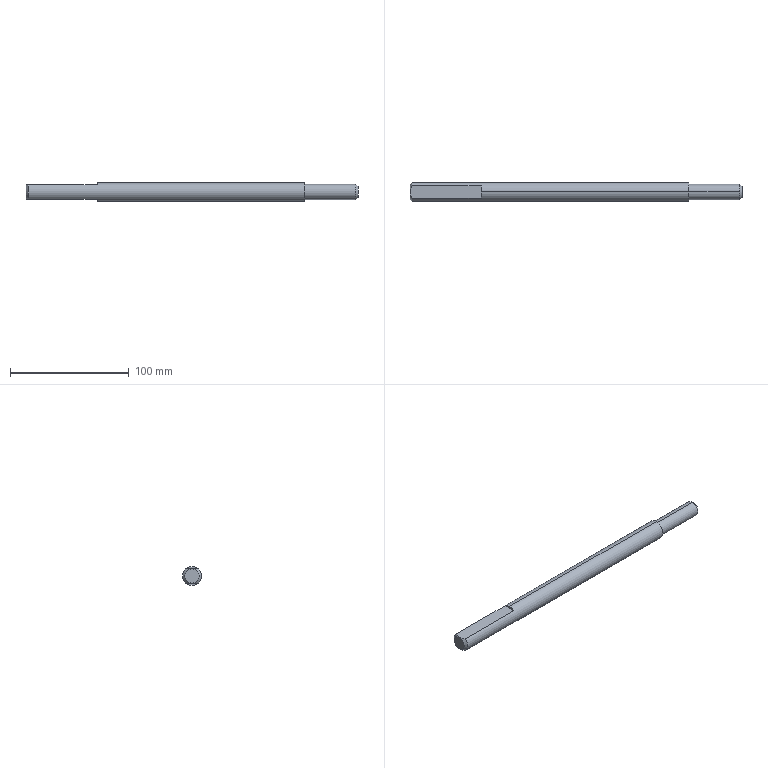Part | SolidWorks | features BaseBody 1 | 1 solid | 15 faces | box 280 x 16 x 16 mm | volume 51352 mm3 | plane 7 | cylinder 4 | cone 4 | commonest cylinder face diameters 13 x2 16 x2
STEP:
#1=CARTESIAN_POINT('',(60.,5.292,6.));
#2=VERTEX_POINT('',#1);
#3=CARTESIAN_POINT('',(60.,0.,8.));
#4=VERTEX_POINT('',#3);
#5=CARTESIAN_POINT('',(60.,0.,0.));
#6=DIRECTION('',(1.,0.,0.));
#7=DIRECTION('',(0.,0.,-1.));
#8=AXIS2_PLACEMENT_3D('',#5,#6,#7);
#9=CIRCLE('',#8,8.);
#10=EDGE_CURVE('',#2,#4,#9,.T.);
#11=ORIENTED_EDGE('',*,*,#10,.T.);
#12=CARTESIAN_POINT('',(235.,0.,8.));
#13=VERTEX_POINT('',#12);
#14=CARTESIAN_POINT('',(117.5,0.,8.));
#15=DIRECTION('',(1.,0.,0.));
#16=VECTOR('',#15,1000.);
#17=LINE('',#14,#16);
#18=EDGE_CURVE('',#4,#13,#17,.T.);
#19=ORIENTED_EDGE('',*,*,#18,.T.);
#20=CARTESIAN_POINT('',(235.,0.,-8.));
#21=VERTEX_POINT('',#20);
#22=CARTESIAN_POINT('',(235.,0.,0.));
#23=DIRECTION('',(-1.,0.,0.));
#24=DIRECTION('',(0.,0.,-1.));
#25=AXIS2_PLACEMENT_3D('',#22,#23,#24);
#26=CIRCLE('',#25,8.);
#27=EDGE_CURVE('',#13,#21,#26,.T.);
#28=ORIENTED_EDGE('',*,*,#27,.T.);
#29=CARTESIAN_POINT('',(60.,0.,-8.));
#30=VERTEX_POINT('',#29);
#31=CARTESIAN_POINT('',(117.5,0.,-8.));
#32=DIRECTION('',(1.,0.,0.));
#33=VECTOR('',#32,1000.);
#34=LINE('',#31,#33);
#35=EDGE_CURVE('',#30,#21,#34,.T.);
#36=ORIENTED_EDGE('',*,*,#35,.F.);
#37=CARTESIAN_POINT('',(60.,5.292,-6.));
#38=VERTEX_POINT('',#37);
#39=CARTESIAN_POINT('',(60.,0.,0.));
#40=DIRECTION('',(1.,0.,0.));
#41=DIRECTION('',(0.,0.,-1.));
#42=AXIS2_PLACEMENT_3D('',#39,#40,#41);
#43=CIRCLE('',#42,8.);
#44=EDGE_CURVE('',#30,#38,#43,.T.);
#45=ORIENTED_EDGE('',*,*,#44,.T.);
#46=CARTESIAN_POINT('',(2.,5.292,-6.));
#47=VERTEX_POINT('',#46);
#48=CARTESIAN_POINT('',(117.5,5.292,-6.));
#49=DIRECTION('',(-1.,0.,0.));
#50=VECTOR('',#49,1000.);
#51=LINE('',#48,#50);
#52=EDGE_CURVE('',#38,#47,#51,.T.);
#53=ORIENTED_EDGE('',*,*,#52,.T.);
#54=CARTESIAN_POINT('',(2.,5.292,6.));
#55=VERTEX_POINT('',#54);
#56=CARTESIAN_POINT('',(2.,0.,0.));
#57=DIRECTION('',(1.,0.,0.));
#58=DIRECTION('',(0.,0.,-1.));
#59=AXIS2_PLACEMENT_3D('',#56,#57,#58);
#60=CIRCLE('',#59,8.);
#61=EDGE_CURVE('',#47,#55,#60,.T.);
#62=ORIENTED_EDGE('',*,*,#61,.T.);
#63=CARTESIAN_POINT('',(117.5,5.292,6.));
#64=DIRECTION('',(1.,0.,0.));
#65=VECTOR('',#64,1000.);
#66=LINE('',#63,#65);
#67=EDGE_CURVE('',#55,#2,#66,.T.);
#68=ORIENTED_EDGE('',*,*,#67,.T.);
#69=EDGE_LOOP('',(#11,#19,#28,#36,#45,#53,#62,#68));
#70=FACE_OUTER_BOUND('',#69,.T.);
#71=CARTESIAN_POINT('',(117.5,0.,0.));
#72=DIRECTION('',(1.,0.,0.));
#73=DIRECTION('',(0.,0.,-1.));
#74=AXIS2_PLACEMENT_3D('',#71,#72,#73);
#75=CYLINDRICAL_SURFACE('',#74,8.);
#76=ADVANCED_FACE('',(#70),#75,.T.);
#77=CARTESIAN_POINT('',(235.,0.,6.5));
#78=VERTEX_POINT('',#77);
#79=CARTESIAN_POINT('',(235.,0.,-6.5));
#80=VERTEX_POINT('',#79);
#81=CARTESIAN_POINT('',(235.,0.,0.));
#82=DIRECTION('',(-1.,0.,0.));
#83=DIRECTION('',(0.,0.,-1.));
#84=AXIS2_PLACEMENT_3D('',#81,#82,#83);
#85=CIRCLE('',#84,6.5);
#86=EDGE_CURVE('',#78,#80,#85,.T.);
#87=ORIENTED_EDGE('',*,*,#86,.F.);
#88=CARTESIAN_POINT('',(278.,0.,6.5));
#89=VERTEX_POINT('',#88);
#90=CARTESIAN_POINT('',(257.5,0.,6.5));
#91=DIRECTION('',(1.,0.,0.));
#92=VECTOR('',#91,1000.);
#93=LINE('',#90,#92);
#94=EDGE_CURVE('',#78,#89,#93,.T.);
#95=ORIENTED_EDGE('',*,*,#94,.T.);
#96=CARTESIAN_POINT('',(278.,0.,-6.5));
#97=VERTEX_POINT('',#96);
#98=CARTESIAN_POINT('',(278.,0.,0.));
#99=DIRECTION('',(-1.,0.,0.));
#100=DIRECTION('',(0.,0.,-1.));
#101=AXIS2_PLACEMENT_3D('',#98,#99,#100);
#102=CIRCLE('',#101,6.5);
#103=EDGE_CURVE('',#89,#97,#102,.T.);
#104=ORIENTED_EDGE('',*,*,#103,.T.);
#105=CARTESIAN_POINT('',(257.5,0.,-6.5));
#106=DIRECTION('',(1.,0.,0.));
#107=VECTOR('',#106,1000.);
#108=LINE('',#105,#107);
#109=EDGE_CURVE('',#80,#97,#108,.T.);
#110=ORIENTED_EDGE('',*,*,#109,.F.);
#111=EDGE_LOOP('',(#87,#95,#104,#110));
#112=FACE_OUTER_BOUND('',#111,.T.);
#113=CARTESIAN_POINT('',(257.5,0.,0.));
#114=DIRECTION('',(1.,0.,0.));
#115=DIRECTION('',(0.,0.,-1.));
#116=AXIS2_PLACEMENT_3D('',#113,#114,#115);
#117=CYLINDRICAL_SURFACE('',#116,6.5);
#118=ADVANCED_FACE('',(#112),#117,.T.);
#119=CARTESIAN_POINT('',(280.,0.,4.5));
#120=VERTEX_POINT('',#119);
#121=CARTESIAN_POINT('',(280.,0.,-4.5));
#122=VERTEX_POINT('',#121);
#123=CARTESIAN_POINT('',(280.,0.,0.));
#124=DIRECTION('',(-1.,0.,0.));
#125=DIRECTION('',(0.,0.,1.));
#126=AXIS2_PLACEMENT_3D('',#123,#124,#125);
#127=CIRCLE('',#126,4.5);
#128=EDGE_CURVE('',#120,#122,#127,.T.);
#129=ORIENTED_EDGE('',*,*,#128,.T.);
#130=CARTESIAN_POINT('',(278.,0.,-6.5));
#131=DIRECTION('',(-0.7071,0.,-0.7071));
#132=VECTOR('',#131,1000.);
#133=LINE('',#130,#132);
#134=EDGE_CURVE('',#122,#97,#133,.T.);
#135=ORIENTED_EDGE('',*,*,#134,.T.);
#136=ORIENTED_EDGE('',*,*,#103,.F.);
#137=CARTESIAN_POINT('',(278.,0.,6.5));
#138=DIRECTION('',(-0.7071,0.,0.7071));
#139=VECTOR('',#138,1000.);
#140=LINE('',#137,#139);
#141=EDGE_CURVE('',#120,#89,#140,.T.);
#142=ORIENTED_EDGE('',*,*,#141,.F.);
#143=EDGE_LOOP('',(#129,#135,#136,#142));
#144=FACE_OUTER_BOUND('',#143,.T.);
#145=CARTESIAN_POINT('',(278.,0.,0.));
#146=DIRECTION('',(-1.,0.,0.));
#147=DIRECTION('',(0.,0.,1.));
#148=AXIS2_PLACEMENT_3D('',#145,#146,#147);
#149=CONICAL_SURFACE('',#148,6.5,0.7854);
#150=ADVANCED_FACE('',(#144),#149,.T.);
#151=ORIENTED_EDGE('',*,*,#18,.F.);
#152=CARTESIAN_POINT('',(60.,-5.292,6.));
#153=VERTEX_POINT('',#152);
#154=CARTESIAN_POINT('',(60.,0.,0.));
#155=DIRECTION('',(1.,0.,0.));
#156=DIRECTION('',(0.,0.,-1.));
#157=AXIS2_PLACEMENT_3D('',#154,#155,#156);
#158=CIRCLE('',#157,8.);
#159=EDGE_CURVE('',#4,#153,#158,.T.);
#160=ORIENTED_EDGE('',*,*,#159,.T.);
#161=CARTESIAN_POINT('',(2.,-5.292,6.));
#162=VERTEX_POINT('',#161);
#163=CARTESIAN_POINT('',(117.5,-5.292,6.));
#164=DIRECTION('',(-1.,0.,0.));
#165=VECTOR('',#164,1000.);
#166=LINE('',#163,#165);
#167=EDGE_CURVE('',#153,#162,#166,.T.);
#168=ORIENTED_EDGE('',*,*,#167,.T.);
#169=CARTESIAN_POINT('',(2.,-5.292,-6.));
#170=VERTEX_POINT('',#169);
#171=CARTESIAN_POINT('',(2.,0.,0.));
#172=DIRECTION('',(1.,0.,0.));
#173=DIRECTION('',(0.,0.,-1.));
#174=AXIS2_PLACEMENT_3D('',#171,#172,#173);
#175=CIRCLE('',#174,8.);
#176=EDGE_CURVE('',#162,#170,#175,.T.);
#177=ORIENTED_EDGE('',*,*,#176,.T.);
#178=CARTESIAN_POINT('',(60.,-5.292,-6.));
#179=VERTEX_POINT('',#178);
#180=CARTESIAN_POINT('',(117.5,-5.292,-6.));
#181=DIRECTION('',(1.,0.,0.));
#182=VECTOR('',#181,1000.);
#183=LINE('',#180,#182);
#184=EDGE_CURVE('',#170,#179,#183,.T.);
#185=ORIENTED_EDGE('',*,*,#184,.T.);
#186=CARTESIAN_POINT('',(60.,0.,0.));
#187=DIRECTION('',(1.,0.,0.));
#188=DIRECTION('',(0.,0.,-1.));
#189=AXIS2_PLACEMENT_3D('',#186,#187,#188);
#190=CIRCLE('',#189,8.);
#191=EDGE_CURVE('',#179,#30,#190,.T.);
#192=ORIENTED_EDGE('',*,*,#191,.T.);
#193=ORIENTED_EDGE('',*,*,#35,.T.);
#194=CARTESIAN_POINT('',(235.,0.,0.));
#195=DIRECTION('',(-1.,0.,0.));
#196=DIRECTION('',(0.,0.,-1.));
#197=AXIS2_PLACEMENT_3D('',#194,#195,#196);
#198=CIRCLE('',#197,8.);
#199=EDGE_CURVE('',#21,#13,#198,.T.);
#200=ORIENTED_EDGE('',*,*,#199,.T.);
#201=EDGE_LOOP('',(#151,#160,#168,#177,#185,#192,#193,#200));
#202=FACE_OUTER_BOUND('',#201,.T.);
#203=CARTESIAN_POINT('',(117.5,0.,0.));
#204=DIRECTION('',(1.,0.,0.));
#205=DIRECTION('',(0.,0.,-1.));
#206=AXIS2_PLACEMENT_3D('',#203,#204,#205);
#207=CYLINDRICAL_SURFACE('',#206,8.);
#208=ADVANCED_FACE('',(#202),#207,.T.);
#209=CARTESIAN_POINT('',(235.,0.,0.));
#210=DIRECTION('',(-1.,0.,0.));
#211=DIRECTION('',(0.,0.,-1.));
#212=AXIS2_PLACEMENT_3D('',#209,#210,#211);
#213=CIRCLE('',#212,6.5);
#214=EDGE_CURVE('',#80,#78,#213,.T.);
#215=ORIENTED_EDGE('',*,*,#214,.T.);
#216=ORIENTED_EDGE('',*,*,#86,.T.);
#217=EDGE_LOOP('',(#215,#216));
#218=FACE_BOUND('',#217,.T.);
#219=ORIENTED_EDGE('',*,*,#199,.F.);
#220=ORIENTED_EDGE('',*,*,#27,.F.);
#221=EDGE_LOOP('',(#219,#220));
#222=FACE_OUTER_BOUND('',#221,.T.);
#223=CARTESIAN_POINT('',(235.,7.25,0.));
#224=DIRECTION('',(1.,0.,0.));
#225=DIRECTION('',(0.,0.,-1.));
#226=AXIS2_PLACEMENT_3D('',#223,#224,#225);
#227=PLANE('',#226);
#228=ADVANCED_FACE('',(#218,#222),#227,.T.);
#229=ORIENTED_EDGE('',*,*,#191,.F.);
#230=CARTESIAN_POINT('',(60.,0.,-6.));
#231=DIRECTION('',(0.,-1.,0.));
#232=VECTOR('',#231,1000.);
#233=LINE('',#230,#232);
#234=EDGE_CURVE('',#38,#179,#233,.T.);
#235=ORIENTED_EDGE('',*,*,#234,.F.);
#236=ORIENTED_EDGE('',*,*,#44,.F.);
#237=EDGE_LOOP('',(#229,#235,#236));
#238=FACE_OUTER_BOUND('',#237,.T.);
#239=CARTESIAN_POINT('',(60.,0.,-6.595));
#240=DIRECTION('',(1.,0.,0.));
#241=DIRECTION('',(0.,0.,-1.));
#242=AXIS2_PLACEMENT_3D('',#239,#240,#241);
#243=PLANE('',#242);
#244=ADVANCED_FACE('',(#238),#243,.F.);
#245=ORIENTED_EDGE('',*,*,#52,.F.);
#246=ORIENTED_EDGE('',*,*,#234,.T.);
#247=ORIENTED_EDGE('',*,*,#184,.F.);
#248=CARTESIAN_POINT('',(0.,0.,-6.));
#249=VERTEX_POINT('',#248);
#250=CARTESIAN_POINT('',(0.,0.,-6.));
#251=CARTESIAN_POINT('',(0.,-0.4837,-6.));
#252=CARTESIAN_POINT('',(0.059,-0.9572,-6.));
#253=CARTESIAN_POINT('',(0.2736,-1.887,-6.));
#254=CARTESIAN_POINT('',(0.4302,-2.347,-6.));
#255=CARTESIAN_POINT('',(0.8016,-3.228,-6.));
#256=CARTESIAN_POINT('',(1.016,-3.654,-6.));
#257=CARTESIAN_POINT('',(1.483,-4.485,-6.));
#258=CARTESIAN_POINT('',(1.736,-4.892,-6.));
#259=CARTESIAN_POINT('',(2.,-5.292,-6.));
#260=B_SPLINE_CURVE_WITH_KNOTS('',3,(#250,#251,#252,#253,#254,#255,#256,#257,#258,#259),.UNSPECIFIED.,.F.,.F.,(4,2,2,2,4),(0.,0.00143,0.00286,0.004289,0.005719),.UNSPECIFIED.);
#261=EDGE_CURVE('',#249,#170,#260,.T.);
#262=ORIENTED_EDGE('',*,*,#261,.F.);
#263=CARTESIAN_POINT('',(2.,5.292,-6.));
#264=CARTESIAN_POINT('',(1.736,4.892,-6.));
#265=CARTESIAN_POINT('',(1.484,4.486,-6.));
#266=CARTESIAN_POINT('',(1.017,3.655,-6.));
#267=CARTESIAN_POINT('',(0.8027,3.23,-6.));
#268=CARTESIAN_POINT('',(0.5246,2.571,-6.));
#269=CARTESIAN_POINT('',(0.4393,2.347,-6.));
#270=CARTESIAN_POINT('',(0.2873,1.891,-6.));
#271=CARTESIAN_POINT('',(0.2209,1.659,-6.));
#272=CARTESIAN_POINT('',(0.05906,0.9584,-6.));
#273=CARTESIAN_POINT('',(0.,0.4839,-6.));
#274=CARTESIAN_POINT('',(0.,0.,-6.));
#275=B_SPLINE_CURVE_WITH_KNOTS('',3,(#263,#264,#265,#266,#267,#268,#269,#270,#271,#272,#273,#274),.UNSPECIFIED.,.F.,.F.,(4,2,2,2,2,4),(0.,0.001428,0.002856,0.003569,0.004283,0.005711),.UNSPECIFIED.);
#276=EDGE_CURVE('',#47,#249,#275,.T.);
#277=ORIENTED_EDGE('',*,*,#276,.F.);
#278=EDGE_LOOP('',(#245,#246,#247,#262,#277));
#279=FACE_OUTER_BOUND('',#278,.T.);
#280=CARTESIAN_POINT('',(0.,5.292,-6.));
#281=DIRECTION('',(0.,0.,1.));
#282=DIRECTION('',(1.,0.,0.));
#283=AXIS2_PLACEMENT_3D('',#280,#281,#282);
#284=PLANE('',#283);
#285=ADVANCED_FACE('',(#279),#284,.F.);
#286=CARTESIAN_POINT('',(0.,0.,6.));
#287=VERTEX_POINT('',#286);
#288=CARTESIAN_POINT('',(2.,-5.292,6.));
#289=CARTESIAN_POINT('',(1.736,-4.892,6.));
#290=CARTESIAN_POINT('',(1.484,-4.486,6.));
#291=CARTESIAN_POINT('',(1.017,-3.655,6.));
#292=CARTESIAN_POINT('',(0.8027,-3.23,6.));
#293=CARTESIAN_POINT('',(0.5246,-2.571,6.));
#294=CARTESIAN_POINT('',(0.4393,-2.347,6.));
#295=CARTESIAN_POINT('',(0.2873,-1.891,6.));
#296=CARTESIAN_POINT('',(0.2209,-1.659,6.));
#297=CARTESIAN_POINT('',(0.05906,-0.9584,6.));
#298=CARTESIAN_POINT('',(0.,-0.4839,6.));
#299=CARTESIAN_POINT('',(0.,0.,6.));
#300=B_SPLINE_CURVE_WITH_KNOTS('',3,(#288,#289,#290,#291,#292,#293,#294,#295,#296,#297,#298,#299),.UNSPECIFIED.,.F.,.F.,(4,2,2,2,2,4),(0.,0.001428,0.002856,0.003569,0.004283,0.005711),.UNSPECIFIED.);
#301=EDGE_CURVE('',#162,#287,#300,.T.);
#302=ORIENTED_EDGE('',*,*,#301,.T.);
#303=CARTESIAN_POINT('',(0.,0.,0.));
#304=DIRECTION('',(1.,0.,0.));
#305=DIRECTION('',(0.,0.,-1.));
#306=AXIS2_PLACEMENT_3D('',#303,#304,#305);
#307=CIRCLE('',#306,6.);
#308=EDGE_CURVE('',#287,#249,#307,.T.);
#309=ORIENTED_EDGE('',*,*,#308,.T.);
#310=ORIENTED_EDGE('',*,*,#261,.T.);
#311=ORIENTED_EDGE('',*,*,#176,.F.);
#312=EDGE_LOOP('',(#302,#309,#310,#311));
#313=FACE_OUTER_BOUND('',#312,.T.);
#314=CARTESIAN_POINT('',(2.,0.,0.));
#315=DIRECTION('',(1.,0.,0.));
#316=DIRECTION('',(0.,0.,-1.));
#317=AXIS2_PLACEMENT_3D('',#314,#315,#316);
#318=CONICAL_SURFACE('',#317,8.,0.7854);
#319=ADVANCED_FACE('',(#313),#318,.T.);
#320=ORIENTED_EDGE('',*,*,#167,.F.);
#321=CARTESIAN_POINT('',(60.,-5.292,6.));
#322=DIRECTION('',(0.,-1.,0.));
#323=VECTOR('',#322,1000.);
#324=LINE('',#321,#323);
#325=EDGE_CURVE('',#2,#153,#324,.T.);
#326=ORIENTED_EDGE('',*,*,#325,.F.);
#327=ORIENTED_EDGE('',*,*,#67,.F.);
#328=CARTESIAN_POINT('',(0.,0.,6.));
#329=CARTESIAN_POINT('',(0.,0.4837,6.));
#330=CARTESIAN_POINT('',(0.059,0.9572,6.));
#331=CARTESIAN_POINT('',(0.2736,1.887,6.));
#332=CARTESIAN_POINT('',(0.4302,2.347,6.));
#333=CARTESIAN_POINT('',(0.8016,3.228,6.));
#334=CARTESIAN_POINT('',(1.016,3.654,6.));
#335=CARTESIAN_POINT('',(1.483,4.485,6.));
#336=CARTESIAN_POINT('',(1.736,4.892,6.));
#337=CARTESIAN_POINT('',(2.,5.292,6.));
#338=B_SPLINE_CURVE_WITH_KNOTS('',3,(#328,#329,#330,#331,#332,#333,#334,#335,#336,#337),.UNSPECIFIED.,.F.,.F.,(4,2,2,2,4),(0.,0.00143,0.00286,0.004289,0.005719),.UNSPECIFIED.);
#339=EDGE_CURVE('',#287,#55,#338,.T.);
#340=ORIENTED_EDGE('',*,*,#339,.F.);
#341=ORIENTED_EDGE('',*,*,#301,.F.);
#342=EDGE_LOOP('',(#320,#326,#327,#340,#341));
#343=FACE_OUTER_BOUND('',#342,.T.);
#344=CARTESIAN_POINT('',(0.,-5.292,6.));
#345=DIRECTION('',(0.,0.,-1.));
#346=DIRECTION('',(0.,1.,0.));
#347=AXIS2_PLACEMENT_3D('',#344,#345,#346);
#348=PLANE('',#347);
#349=ADVANCED_FACE('',(#343),#348,.F.);
#350=ORIENTED_EDGE('',*,*,#10,.F.);
#351=ORIENTED_EDGE('',*,*,#325,.T.);
#352=ORIENTED_EDGE('',*,*,#159,.F.);
#353=EDGE_LOOP('',(#350,#351,#352));
#354=FACE_OUTER_BOUND('',#353,.T.);
#355=CARTESIAN_POINT('',(60.,0.,6.595));
#356=DIRECTION('',(1.,0.,0.));
#357=DIRECTION('',(0.,0.,-1.));
#358=AXIS2_PLACEMENT_3D('',#355,#356,#357);
#359=PLANE('',#358);
#360=ADVANCED_FACE('',(#354),#359,.F.);
#361=ORIENTED_EDGE('',*,*,#339,.T.);
#362=ORIENTED_EDGE('',*,*,#61,.F.);
#363=ORIENTED_EDGE('',*,*,#276,.T.);
#364=CARTESIAN_POINT('',(0.,0.,0.));
#365=DIRECTION('',(1.,0.,0.));
#366=DIRECTION('',(0.,0.,-1.));
#367=AXIS2_PLACEMENT_3D('',#364,#365,#366);
#368=CIRCLE('',#367,6.);
#369=EDGE_CURVE('',#249,#287,#368,.T.);
#370=ORIENTED_EDGE('',*,*,#369,.T.);
#371=EDGE_LOOP('',(#361,#362,#363,#370));
#372=FACE_OUTER_BOUND('',#371,.T.);
#373=CARTESIAN_POINT('',(2.,0.,0.));
#374=DIRECTION('',(1.,0.,0.));
#375=DIRECTION('',(0.,0.,-1.));
#376=AXIS2_PLACEMENT_3D('',#373,#374,#375);
#377=CONICAL_SURFACE('',#376,8.,0.7854);
#378=ADVANCED_FACE('',(#372),#377,.T.);
#379=ORIENTED_EDGE('',*,*,#94,.F.);
#380=ORIENTED_EDGE('',*,*,#214,.F.);
#381=ORIENTED_EDGE('',*,*,#109,.T.);
#382=CARTESIAN_POINT('',(278.,0.,0.));
#383=DIRECTION('',(-1.,0.,0.));
#384=DIRECTION('',(0.,0.,-1.));
#385=AXIS2_PLACEMENT_3D('',#382,#383,#384);
#386=CIRCLE('',#385,6.5);
#387=EDGE_CURVE('',#97,#89,#386,.T.);
#388=ORIENTED_EDGE('',*,*,#387,.T.);
#389=EDGE_LOOP('',(#379,#380,#381,#388));
#390=FACE_OUTER_BOUND('',#389,.T.);
#391=CARTESIAN_POINT('',(257.5,0.,0.));
#392=DIRECTION('',(1.,0.,0.));
#393=DIRECTION('',(0.,0.,-1.));
#394=AXIS2_PLACEMENT_3D('',#391,#392,#393);
#395=CYLINDRICAL_SURFACE('',#394,6.5);
#396=ADVANCED_FACE('',(#390),#395,.T.);
#397=ORIENTED_EDGE('',*,*,#369,.F.);
#398=ORIENTED_EDGE('',*,*,#308,.F.);
#399=EDGE_LOOP('',(#397,#398));
#400=FACE_OUTER_BOUND('',#399,.T.);
#401=CARTESIAN_POINT('',(0.,4.,0.));
#402=DIRECTION('',(-1.,0.,0.));
#403=DIRECTION('',(0.,0.,1.));
#404=AXIS2_PLACEMENT_3D('',#401,#402,#403);
#405=PLANE('',#404);
#406=ADVANCED_FACE('',(#400),#405,.T.);
#407=ORIENTED_EDGE('',*,*,#134,.F.);
#408=CARTESIAN_POINT('',(280.,0.,0.));
#409=DIRECTION('',(-1.,0.,0.));
#410=DIRECTION('',(0.,0.,1.));
#411=AXIS2_PLACEMENT_3D('',#408,#409,#410);
#412=CIRCLE('',#411,4.5);
#413=EDGE_CURVE('',#122,#120,#412,.T.);
#414=ORIENTED_EDGE('',*,*,#413,.T.);
#415=ORIENTED_EDGE('',*,*,#141,.T.);
#416=ORIENTED_EDGE('',*,*,#387,.F.);
#417=EDGE_LOOP('',(#407,#414,#415,#416));
#418=FACE_OUTER_BOUND('',#417,.T.);
#419=CARTESIAN_POINT('',(278.,0.,0.));
#420=DIRECTION('',(-1.,0.,0.));
#421=DIRECTION('',(0.,0.,1.));
#422=AXIS2_PLACEMENT_3D('',#419,#420,#421);
#423=CONICAL_SURFACE('',#422,6.5,0.7854);
#424=ADVANCED_FACE('',(#418),#423,.T.);
#425=ORIENTED_EDGE('',*,*,#128,.F.);
#426=ORIENTED_EDGE('',*,*,#413,.F.);
#427=EDGE_LOOP('',(#425,#426));
#428=FACE_OUTER_BOUND('',#427,.T.);
#429=CARTESIAN_POINT('',(280.,3.25,0.));
#430=DIRECTION('',(1.,0.,0.));
#431=DIRECTION('',(0.,0.,-1.));
#432=AXIS2_PLACEMENT_3D('',#429,#430,#431);
#433=PLANE('',#432);
#434=ADVANCED_FACE('',(#428),#433,.T.);
#435=CLOSED_SHELL('',(#76,#118,#150,#208,#228,#244,#285,#319,#349,#360,#378,#396,#406,#424,#434));
#436=MANIFOLD_SOLID_BREP('',#435);
#437=CARTESIAN_POINT('',(0.,0.,0.));
#438=DIRECTION('',(0.,0.,1.));
#439=DIRECTION('',(1.,0.,0.));
#440=AXIS2_PLACEMENT_3D('',#437,#438,#439);
#441=(LENGTH_UNIT()NAMED_UNIT(*)SI_UNIT(.MILLI.,.METRE.));
#442=UNCERTAINTY_MEASURE_WITH_UNIT(LENGTH_MEASURE(0.00001),#441,'','');
#443=(NAMED_UNIT(*)PLANE_ANGLE_UNIT()SI_UNIT($,.RADIAN.));
#444=(NAMED_UNIT(*)SI_UNIT($,.STERADIAN.)SOLID_ANGLE_UNIT());
#445=(GEOMETRIC_REPRESENTATION_CONTEXT(3)GLOBAL_UNCERTAINTY_ASSIGNED_CONTEXT((#442))GLOBAL_UNIT_ASSIGNED_CONTEXT((#441,#443,#444))REPRESENTATION_CONTEXT('',''));
#446=ADVANCED_BREP_SHAPE_REPRESENTATION('',(#436,#440),#445);